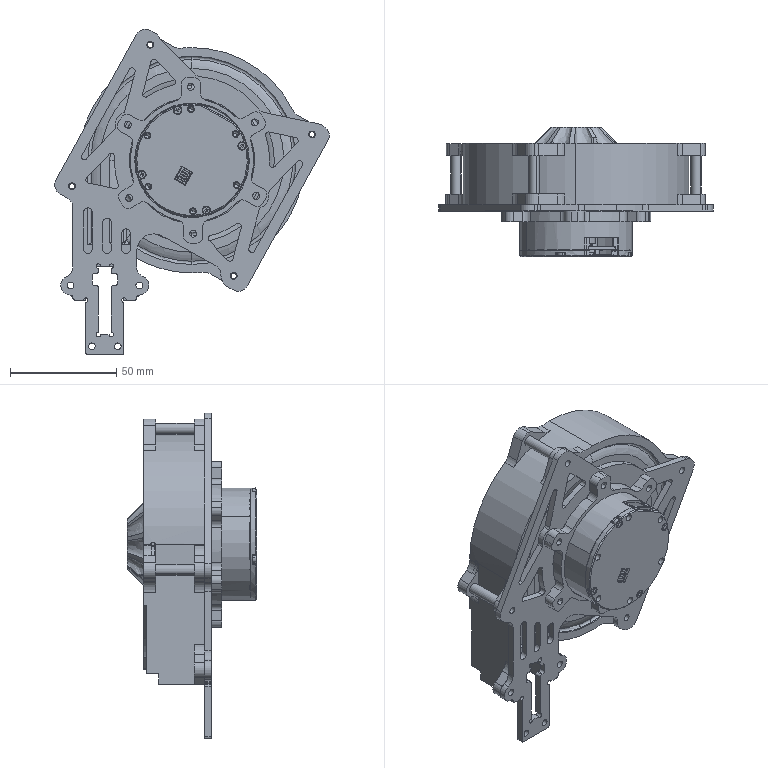Part | SolidWorks | features CompositeCurve 40 | 64 solids | 2628 faces | box 129.15 x 61 x 153.15 mm | volume 192144 mm3 | cylinder 1284 | plane 758 | torus 268 | cone 213 | spline 105 | commonest cylinder face diameters 4 x170 2 x149 2.7 x72 4.4 x60 3.2 x56 5 x56